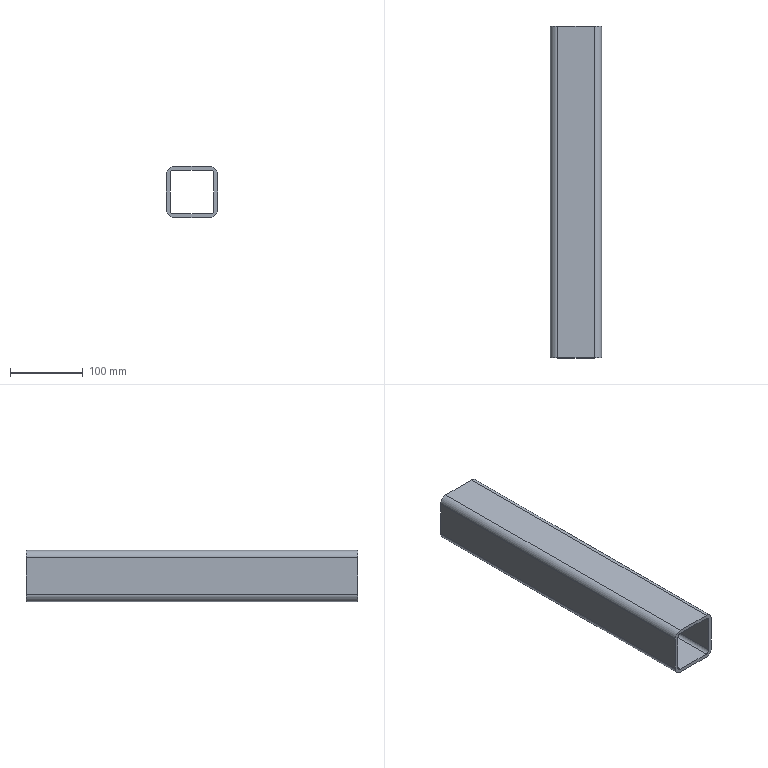Part | SolidWorks | features WeldMemberFeat 1, WeldmentFeature 1 | 1 solid | 18 faces | box 70 x 455 x 70 mm | volume 562207 mm3 | plane 10 | cylinder 8 | commonest cylinder face diameters 10 x4 20 x4
STEP:
#1=CARTESIAN_POINT('',(-35.,0.,25.));
#2=VERTEX_POINT('',#1);
#3=CARTESIAN_POINT('',(-25.,0.,35.));
#4=VERTEX_POINT('',#3);
#5=CARTESIAN_POINT('',(-25.,0.,25.));
#6=DIRECTION('',(0.,1.,0.));
#7=DIRECTION('',(0.,0.,1.));
#8=AXIS2_PLACEMENT_3D('',#5,#6,#7);
#9=CIRCLE('',#8,10.);
#10=EDGE_CURVE('',#2,#4,#9,.T.);
#11=ORIENTED_EDGE('',*,*,#10,.T.);
#12=CARTESIAN_POINT('',(-25.,455.,35.));
#13=VERTEX_POINT('',#12);
#14=CARTESIAN_POINT('',(-25.,455.,35.));
#15=DIRECTION('',(0.,-1.,0.));
#16=VECTOR('',#15,1000.);
#17=LINE('',#14,#16);
#18=EDGE_CURVE('',#13,#4,#17,.T.);
#19=ORIENTED_EDGE('',*,*,#18,.F.);
#20=CARTESIAN_POINT('',(-35.,455.,25.));
#21=VERTEX_POINT('',#20);
#22=CARTESIAN_POINT('',(-25.,455.,25.));
#23=DIRECTION('',(0.,1.,0.));
#24=DIRECTION('',(0.,0.,1.));
#25=AXIS2_PLACEMENT_3D('',#22,#23,#24);
#26=CIRCLE('',#25,10.);
#27=EDGE_CURVE('',#21,#13,#26,.T.);
#28=ORIENTED_EDGE('',*,*,#27,.F.);
#29=CARTESIAN_POINT('',(-35.,455.,25.));
#30=DIRECTION('',(0.,-1.,0.));
#31=VECTOR('',#30,1000.);
#32=LINE('',#29,#31);
#33=EDGE_CURVE('',#21,#2,#32,.T.);
#34=ORIENTED_EDGE('',*,*,#33,.T.);
#35=EDGE_LOOP('',(#11,#19,#28,#34));
#36=FACE_OUTER_BOUND('',#35,.T.);
#37=CARTESIAN_POINT('',(-25.,455.,25.));
#38=DIRECTION('',(0.,-1.,0.));
#39=DIRECTION('',(0.,0.,-1.));
#40=AXIS2_PLACEMENT_3D('',#37,#38,#39);
#41=CYLINDRICAL_SURFACE('',#40,10.);
#42=ADVANCED_FACE('',(#36),#41,.T.);
#43=CARTESIAN_POINT('',(25.,0.,35.));
#44=VERTEX_POINT('',#43);
#45=CARTESIAN_POINT('',(-25.,0.,35.));
#46=DIRECTION('',(1.,0.,0.));
#47=VECTOR('',#46,1000.);
#48=LINE('',#45,#47);
#49=EDGE_CURVE('',#4,#44,#48,.T.);
#50=ORIENTED_EDGE('',*,*,#49,.T.);
#51=CARTESIAN_POINT('',(25.,455.,35.));
#52=VERTEX_POINT('',#51);
#53=CARTESIAN_POINT('',(25.,455.,35.));
#54=DIRECTION('',(0.,-1.,0.));
#55=VECTOR('',#54,1000.);
#56=LINE('',#53,#55);
#57=EDGE_CURVE('',#52,#44,#56,.T.);
#58=ORIENTED_EDGE('',*,*,#57,.F.);
#59=CARTESIAN_POINT('',(-25.,455.,35.));
#60=DIRECTION('',(1.,0.,0.));
#61=VECTOR('',#60,1000.);
#62=LINE('',#59,#61);
#63=EDGE_CURVE('',#13,#52,#62,.T.);
#64=ORIENTED_EDGE('',*,*,#63,.F.);
#65=ORIENTED_EDGE('',*,*,#18,.T.);
#66=EDGE_LOOP('',(#50,#58,#64,#65));
#67=FACE_OUTER_BOUND('',#66,.T.);
#68=CARTESIAN_POINT('',(-25.,455.,35.));
#69=DIRECTION('',(0.,0.,-1.));
#70=DIRECTION('',(-1.,0.,0.));
#71=AXIS2_PLACEMENT_3D('',#68,#69,#70);
#72=PLANE('',#71);
#73=ADVANCED_FACE('',(#67),#72,.F.);
#74=CARTESIAN_POINT('',(35.,0.,25.));
#75=VERTEX_POINT('',#74);
#76=CARTESIAN_POINT('',(25.,0.,25.));
#77=DIRECTION('',(0.,1.,0.));
#78=DIRECTION('',(0.,0.,1.));
#79=AXIS2_PLACEMENT_3D('',#76,#77,#78);
#80=CIRCLE('',#79,10.);
#81=EDGE_CURVE('',#44,#75,#80,.T.);
#82=ORIENTED_EDGE('',*,*,#81,.T.);
#83=CARTESIAN_POINT('',(35.,455.,25.));
#84=VERTEX_POINT('',#83);
#85=CARTESIAN_POINT('',(35.,455.,25.));
#86=DIRECTION('',(0.,-1.,0.));
#87=VECTOR('',#86,1000.);
#88=LINE('',#85,#87);
#89=EDGE_CURVE('',#84,#75,#88,.T.);
#90=ORIENTED_EDGE('',*,*,#89,.F.);
#91=CARTESIAN_POINT('',(25.,455.,25.));
#92=DIRECTION('',(0.,1.,0.));
#93=DIRECTION('',(0.,0.,1.));
#94=AXIS2_PLACEMENT_3D('',#91,#92,#93);
#95=CIRCLE('',#94,10.);
#96=EDGE_CURVE('',#52,#84,#95,.T.);
#97=ORIENTED_EDGE('',*,*,#96,.F.);
#98=ORIENTED_EDGE('',*,*,#57,.T.);
#99=EDGE_LOOP('',(#82,#90,#97,#98));
#100=FACE_OUTER_BOUND('',#99,.T.);
#101=CARTESIAN_POINT('',(25.,455.,25.));
#102=DIRECTION('',(0.,-1.,0.));
#103=DIRECTION('',(0.,0.,-1.));
#104=AXIS2_PLACEMENT_3D('',#101,#102,#103);
#105=CYLINDRICAL_SURFACE('',#104,10.);
#106=ADVANCED_FACE('',(#100),#105,.T.);
#107=CARTESIAN_POINT('',(35.,0.,-25.));
#108=VERTEX_POINT('',#107);
#109=CARTESIAN_POINT('',(35.,0.,-25.));
#110=DIRECTION('',(0.,0.,-1.));
#111=VECTOR('',#110,1000.);
#112=LINE('',#109,#111);
#113=EDGE_CURVE('',#75,#108,#112,.T.);
#114=ORIENTED_EDGE('',*,*,#113,.T.);
#115=CARTESIAN_POINT('',(35.,455.,-25.));
#116=VERTEX_POINT('',#115);
#117=CARTESIAN_POINT('',(35.,455.,-25.));
#118=DIRECTION('',(0.,-1.,0.));
#119=VECTOR('',#118,1000.);
#120=LINE('',#117,#119);
#121=EDGE_CURVE('',#116,#108,#120,.T.);
#122=ORIENTED_EDGE('',*,*,#121,.F.);
#123=CARTESIAN_POINT('',(35.,455.,-25.));
#124=DIRECTION('',(0.,0.,-1.));
#125=VECTOR('',#124,1000.);
#126=LINE('',#123,#125);
#127=EDGE_CURVE('',#84,#116,#126,.T.);
#128=ORIENTED_EDGE('',*,*,#127,.F.);
#129=ORIENTED_EDGE('',*,*,#89,.T.);
#130=EDGE_LOOP('',(#114,#122,#128,#129));
#131=FACE_OUTER_BOUND('',#130,.T.);
#132=CARTESIAN_POINT('',(35.,455.,-25.));
#133=DIRECTION('',(-1.,0.,0.));
#134=DIRECTION('',(0.,0.,1.));
#135=AXIS2_PLACEMENT_3D('',#132,#133,#134);
#136=PLANE('',#135);
#137=ADVANCED_FACE('',(#131),#136,.F.);
#138=CARTESIAN_POINT('',(25.,0.,-35.));
#139=VERTEX_POINT('',#138);
#140=CARTESIAN_POINT('',(25.,0.,-25.));
#141=DIRECTION('',(0.,1.,0.));
#142=DIRECTION('',(0.,0.,1.));
#143=AXIS2_PLACEMENT_3D('',#140,#141,#142);
#144=CIRCLE('',#143,10.);
#145=EDGE_CURVE('',#108,#139,#144,.T.);
#146=ORIENTED_EDGE('',*,*,#145,.T.);
#147=CARTESIAN_POINT('',(25.,455.,-35.));
#148=VERTEX_POINT('',#147);
#149=CARTESIAN_POINT('',(25.,455.,-35.));
#150=DIRECTION('',(0.,-1.,0.));
#151=VECTOR('',#150,1000.);
#152=LINE('',#149,#151);
#153=EDGE_CURVE('',#148,#139,#152,.T.);
#154=ORIENTED_EDGE('',*,*,#153,.F.);
#155=CARTESIAN_POINT('',(25.,455.,-25.));
#156=DIRECTION('',(0.,1.,0.));
#157=DIRECTION('',(0.,0.,1.));
#158=AXIS2_PLACEMENT_3D('',#155,#156,#157);
#159=CIRCLE('',#158,10.);
#160=EDGE_CURVE('',#116,#148,#159,.T.);
#161=ORIENTED_EDGE('',*,*,#160,.F.);
#162=ORIENTED_EDGE('',*,*,#121,.T.);
#163=EDGE_LOOP('',(#146,#154,#161,#162));
#164=FACE_OUTER_BOUND('',#163,.T.);
#165=CARTESIAN_POINT('',(25.,455.,-25.));
#166=DIRECTION('',(0.,-1.,0.));
#167=DIRECTION('',(0.,0.,-1.));
#168=AXIS2_PLACEMENT_3D('',#165,#166,#167);
#169=CYLINDRICAL_SURFACE('',#168,10.);
#170=ADVANCED_FACE('',(#164),#169,.T.);
#171=CARTESIAN_POINT('',(-25.,0.,-35.));
#172=VERTEX_POINT('',#171);
#173=CARTESIAN_POINT('',(25.,0.,-35.));
#174=DIRECTION('',(-1.,0.,0.));
#175=VECTOR('',#174,1000.);
#176=LINE('',#173,#175);
#177=EDGE_CURVE('',#139,#172,#176,.T.);
#178=ORIENTED_EDGE('',*,*,#177,.T.);
#179=CARTESIAN_POINT('',(-25.,455.,-35.));
#180=VERTEX_POINT('',#179);
#181=CARTESIAN_POINT('',(-25.,455.,-35.));
#182=DIRECTION('',(0.,-1.,0.));
#183=VECTOR('',#182,1000.);
#184=LINE('',#181,#183);
#185=EDGE_CURVE('',#180,#172,#184,.T.);
#186=ORIENTED_EDGE('',*,*,#185,.F.);
#187=CARTESIAN_POINT('',(25.,455.,-35.));
#188=DIRECTION('',(-1.,0.,0.));
#189=VECTOR('',#188,1000.);
#190=LINE('',#187,#189);
#191=EDGE_CURVE('',#148,#180,#190,.T.);
#192=ORIENTED_EDGE('',*,*,#191,.F.);
#193=ORIENTED_EDGE('',*,*,#153,.T.);
#194=EDGE_LOOP('',(#178,#186,#192,#193));
#195=FACE_OUTER_BOUND('',#194,.T.);
#196=CARTESIAN_POINT('',(25.,455.,-35.));
#197=DIRECTION('',(0.,0.,1.));
#198=DIRECTION('',(1.,0.,0.));
#199=AXIS2_PLACEMENT_3D('',#196,#197,#198);
#200=PLANE('',#199);
#201=ADVANCED_FACE('',(#195),#200,.F.);
#202=CARTESIAN_POINT('',(-35.,0.,-25.));
#203=VERTEX_POINT('',#202);
#204=CARTESIAN_POINT('',(-25.,0.,-25.));
#205=DIRECTION('',(0.,1.,0.));
#206=DIRECTION('',(0.,0.,1.));
#207=AXIS2_PLACEMENT_3D('',#204,#205,#206);
#208=CIRCLE('',#207,10.);
#209=EDGE_CURVE('',#172,#203,#208,.T.);
#210=ORIENTED_EDGE('',*,*,#209,.T.);
#211=CARTESIAN_POINT('',(-35.,455.,-25.));
#212=VERTEX_POINT('',#211);
#213=CARTESIAN_POINT('',(-35.,455.,-25.));
#214=DIRECTION('',(0.,-1.,0.));
#215=VECTOR('',#214,1000.);
#216=LINE('',#213,#215);
#217=EDGE_CURVE('',#212,#203,#216,.T.);
#218=ORIENTED_EDGE('',*,*,#217,.F.);
#219=CARTESIAN_POINT('',(-25.,455.,-25.));
#220=DIRECTION('',(0.,1.,0.));
#221=DIRECTION('',(0.,0.,1.));
#222=AXIS2_PLACEMENT_3D('',#219,#220,#221);
#223=CIRCLE('',#222,10.);
#224=EDGE_CURVE('',#180,#212,#223,.T.);
#225=ORIENTED_EDGE('',*,*,#224,.F.);
#226=ORIENTED_EDGE('',*,*,#185,.T.);
#227=EDGE_LOOP('',(#210,#218,#225,#226));
#228=FACE_OUTER_BOUND('',#227,.T.);
#229=CARTESIAN_POINT('',(-25.,455.,-25.));
#230=DIRECTION('',(0.,-1.,0.));
#231=DIRECTION('',(0.,0.,-1.));
#232=AXIS2_PLACEMENT_3D('',#229,#230,#231);
#233=CYLINDRICAL_SURFACE('',#232,10.);
#234=ADVANCED_FACE('',(#228),#233,.T.);
#235=CARTESIAN_POINT('',(25.,0.,30.));
#236=VERTEX_POINT('',#235);
#237=CARTESIAN_POINT('',(30.,0.,25.));
#238=VERTEX_POINT('',#237);
#239=CARTESIAN_POINT('',(25.,0.,25.));
#240=DIRECTION('',(0.,1.,0.));
#241=DIRECTION('',(0.,0.,1.));
#242=AXIS2_PLACEMENT_3D('',#239,#240,#241);
#243=CIRCLE('',#242,5.);
#244=EDGE_CURVE('',#236,#238,#243,.T.);
#245=ORIENTED_EDGE('',*,*,#244,.F.);
#246=CARTESIAN_POINT('',(25.,455.,30.));
#247=VERTEX_POINT('',#246);
#248=CARTESIAN_POINT('',(25.,455.,30.));
#249=DIRECTION('',(0.,-1.,0.));
#250=VECTOR('',#249,1000.);
#251=LINE('',#248,#250);
#252=EDGE_CURVE('',#247,#236,#251,.T.);
#253=ORIENTED_EDGE('',*,*,#252,.F.);
#254=CARTESIAN_POINT('',(30.,455.,25.));
#255=VERTEX_POINT('',#254);
#256=CARTESIAN_POINT('',(25.,455.,25.));
#257=DIRECTION('',(0.,1.,0.));
#258=DIRECTION('',(0.,0.,1.));
#259=AXIS2_PLACEMENT_3D('',#256,#257,#258);
#260=CIRCLE('',#259,5.);
#261=EDGE_CURVE('',#247,#255,#260,.T.);
#262=ORIENTED_EDGE('',*,*,#261,.T.);
#263=CARTESIAN_POINT('',(30.,455.,25.));
#264=DIRECTION('',(0.,-1.,0.));
#265=VECTOR('',#264,1000.);
#266=LINE('',#263,#265);
#267=EDGE_CURVE('',#255,#238,#266,.T.);
#268=ORIENTED_EDGE('',*,*,#267,.T.);
#269=EDGE_LOOP('',(#245,#253,#262,#268));
#270=FACE_OUTER_BOUND('',#269,.T.);
#271=CARTESIAN_POINT('',(25.,455.,25.));
#272=DIRECTION('',(0.,-1.,0.));
#273=DIRECTION('',(0.,0.,-1.));
#274=AXIS2_PLACEMENT_3D('',#271,#272,#273);
#275=CYLINDRICAL_SURFACE('',#274,5.);
#276=ADVANCED_FACE('',(#270),#275,.F.);
#277=CARTESIAN_POINT('',(-25.,0.,30.));
#278=VERTEX_POINT('',#277);
#279=CARTESIAN_POINT('',(-25.,0.,30.));
#280=DIRECTION('',(1.,0.,0.));
#281=VECTOR('',#280,1000.);
#282=LINE('',#279,#281);
#283=EDGE_CURVE('',#278,#236,#282,.T.);
#284=ORIENTED_EDGE('',*,*,#283,.F.);
#285=CARTESIAN_POINT('',(-25.,455.,30.));
#286=VERTEX_POINT('',#285);
#287=CARTESIAN_POINT('',(-25.,455.,30.));
#288=DIRECTION('',(0.,-1.,0.));
#289=VECTOR('',#288,1000.);
#290=LINE('',#287,#289);
#291=EDGE_CURVE('',#286,#278,#290,.T.);
#292=ORIENTED_EDGE('',*,*,#291,.F.);
#293=CARTESIAN_POINT('',(-25.,455.,30.));
#294=DIRECTION('',(1.,0.,0.));
#295=VECTOR('',#294,1000.);
#296=LINE('',#293,#295);
#297=EDGE_CURVE('',#286,#247,#296,.T.);
#298=ORIENTED_EDGE('',*,*,#297,.T.);
#299=ORIENTED_EDGE('',*,*,#252,.T.);
#300=EDGE_LOOP('',(#284,#292,#298,#299));
#301=FACE_OUTER_BOUND('',#300,.T.);
#302=CARTESIAN_POINT('',(-25.,455.,30.));
#303=DIRECTION('',(0.,0.,-1.));
#304=DIRECTION('',(-1.,0.,0.));
#305=AXIS2_PLACEMENT_3D('',#302,#303,#304);
#306=PLANE('',#305);
#307=ADVANCED_FACE('',(#301),#306,.T.);
#308=CARTESIAN_POINT('',(-30.,0.,25.));
#309=VERTEX_POINT('',#308);
#310=CARTESIAN_POINT('',(-25.,0.,25.));
#311=DIRECTION('',(0.,1.,0.));
#312=DIRECTION('',(0.,0.,1.));
#313=AXIS2_PLACEMENT_3D('',#310,#311,#312);
#314=CIRCLE('',#313,5.);
#315=EDGE_CURVE('',#309,#278,#314,.T.);
#316=ORIENTED_EDGE('',*,*,#315,.F.);
#317=CARTESIAN_POINT('',(-30.,455.,25.));
#318=VERTEX_POINT('',#317);
#319=CARTESIAN_POINT('',(-30.,455.,25.));
#320=DIRECTION('',(0.,-1.,0.));
#321=VECTOR('',#320,1000.);
#322=LINE('',#319,#321);
#323=EDGE_CURVE('',#318,#309,#322,.T.);
#324=ORIENTED_EDGE('',*,*,#323,.F.);
#325=CARTESIAN_POINT('',(-25.,455.,25.));
#326=DIRECTION('',(0.,1.,0.));
#327=DIRECTION('',(0.,0.,1.));
#328=AXIS2_PLACEMENT_3D('',#325,#326,#327);
#329=CIRCLE('',#328,5.);
#330=EDGE_CURVE('',#318,#286,#329,.T.);
#331=ORIENTED_EDGE('',*,*,#330,.T.);
#332=ORIENTED_EDGE('',*,*,#291,.T.);
#333=EDGE_LOOP('',(#316,#324,#331,#332));
#334=FACE_OUTER_BOUND('',#333,.T.);
#335=CARTESIAN_POINT('',(-25.,455.,25.));
#336=DIRECTION('',(0.,-1.,0.));
#337=DIRECTION('',(0.,0.,-1.));
#338=AXIS2_PLACEMENT_3D('',#335,#336,#337);
#339=CYLINDRICAL_SURFACE('',#338,5.);
#340=ADVANCED_FACE('',(#334),#339,.F.);
#341=CARTESIAN_POINT('',(-30.,0.,-25.));
#342=VERTEX_POINT('',#341);
#343=CARTESIAN_POINT('',(-30.,0.,25.));
#344=DIRECTION('',(0.,0.,1.));
#345=VECTOR('',#344,1000.);
#346=LINE('',#343,#345);
#347=EDGE_CURVE('',#342,#309,#346,.T.);
#348=ORIENTED_EDGE('',*,*,#347,.F.);
#349=CARTESIAN_POINT('',(-30.,455.,-25.));
#350=VERTEX_POINT('',#349);
#351=CARTESIAN_POINT('',(-30.,455.,-25.));
#352=DIRECTION('',(0.,-1.,0.));
#353=VECTOR('',#352,1000.);
#354=LINE('',#351,#353);
#355=EDGE_CURVE('',#350,#342,#354,.T.);
#356=ORIENTED_EDGE('',*,*,#355,.F.);
#357=CARTESIAN_POINT('',(-30.,455.,25.));
#358=DIRECTION('',(0.,0.,1.));
#359=VECTOR('',#358,1000.);
#360=LINE('',#357,#359);
#361=EDGE_CURVE('',#350,#318,#360,.T.);
#362=ORIENTED_EDGE('',*,*,#361,.T.);
#363=ORIENTED_EDGE('',*,*,#323,.T.);
#364=EDGE_LOOP('',(#348,#356,#362,#363));
#365=FACE_OUTER_BOUND('',#364,.T.);
#366=CARTESIAN_POINT('',(-30.,455.,25.));
#367=DIRECTION('',(1.,0.,0.));
#368=DIRECTION('',(0.,0.,-1.));
#369=AXIS2_PLACEMENT_3D('',#366,#367,#368);
#370=PLANE('',#369);
#371=ADVANCED_FACE('',(#365),#370,.T.);
#372=CARTESIAN_POINT('',(-25.,0.,-30.));
#373=VERTEX_POINT('',#372);
#374=CARTESIAN_POINT('',(-25.,0.,-25.));
#375=DIRECTION('',(0.,1.,0.));
#376=DIRECTION('',(0.,0.,1.));
#377=AXIS2_PLACEMENT_3D('',#374,#375,#376);
#378=CIRCLE('',#377,5.);
#379=EDGE_CURVE('',#373,#342,#378,.T.);
#380=ORIENTED_EDGE('',*,*,#379,.F.);
#381=CARTESIAN_POINT('',(-25.,455.,-30.));
#382=VERTEX_POINT('',#381);
#383=CARTESIAN_POINT('',(-25.,455.,-30.));
#384=DIRECTION('',(0.,-1.,0.));
#385=VECTOR('',#384,1000.);
#386=LINE('',#383,#385);
#387=EDGE_CURVE('',#382,#373,#386,.T.);
#388=ORIENTED_EDGE('',*,*,#387,.F.);
#389=CARTESIAN_POINT('',(-25.,455.,-25.));
#390=DIRECTION('',(0.,1.,0.));
#391=DIRECTION('',(0.,0.,1.));
#392=AXIS2_PLACEMENT_3D('',#389,#390,#391);
#393=CIRCLE('',#392,5.);
#394=EDGE_CURVE('',#382,#350,#393,.T.);
#395=ORIENTED_EDGE('',*,*,#394,.T.);
#396=ORIENTED_EDGE('',*,*,#355,.T.);
#397=EDGE_LOOP('',(#380,#388,#395,#396));
#398=FACE_OUTER_BOUND('',#397,.T.);
#399=CARTESIAN_POINT('',(-25.,455.,-25.));
#400=DIRECTION('',(0.,-1.,0.));
#401=DIRECTION('',(0.,0.,-1.));
#402=AXIS2_PLACEMENT_3D('',#399,#400,#401);
#403=CYLINDRICAL_SURFACE('',#402,5.);
#404=ADVANCED_FACE('',(#398),#403,.F.);
#405=CARTESIAN_POINT('',(25.,0.,-30.));
#406=VERTEX_POINT('',#405);
#407=CARTESIAN_POINT('',(25.,0.,-30.));
#408=DIRECTION('',(-1.,0.,0.));
#409=VECTOR('',#408,1000.);
#410=LINE('',#407,#409);
#411=EDGE_CURVE('',#406,#373,#410,.T.);
#412=ORIENTED_EDGE('',*,*,#411,.F.);
#413=CARTESIAN_POINT('',(25.,455.,-30.));
#414=VERTEX_POINT('',#413);
#415=CARTESIAN_POINT('',(25.,455.,-30.));
#416=DIRECTION('',(0.,-1.,0.));
#417=VECTOR('',#416,1000.);
#418=LINE('',#415,#417);
#419=EDGE_CURVE('',#414,#406,#418,.T.);
#420=ORIENTED_EDGE('',*,*,#419,.F.);
#421=CARTESIAN_POINT('',(25.,455.,-30.));
#422=DIRECTION('',(-1.,0.,0.));
#423=VECTOR('',#422,1000.);
#424=LINE('',#421,#423);
#425=EDGE_CURVE('',#414,#382,#424,.T.);
#426=ORIENTED_EDGE('',*,*,#425,.T.);
#427=ORIENTED_EDGE('',*,*,#387,.T.);
#428=EDGE_LOOP('',(#412,#420,#426,#427));
#429=FACE_OUTER_BOUND('',#428,.T.);
#430=CARTESIAN_POINT('',(25.,455.,-30.));
#431=DIRECTION('',(0.,0.,1.));
#432=DIRECTION('',(1.,0.,0.));
#433=AXIS2_PLACEMENT_3D('',#430,#431,#432);
#434=PLANE('',#433);
#435=ADVANCED_FACE('',(#429),#434,.T.);
#436=CARTESIAN_POINT('',(30.,0.,-25.));
#437=VERTEX_POINT('',#436);
#438=CARTESIAN_POINT('',(25.,0.,-25.));
#439=DIRECTION('',(0.,1.,0.));
#440=DIRECTION('',(0.,0.,1.));
#441=AXIS2_PLACEMENT_3D('',#438,#439,#440);
#442=CIRCLE('',#441,5.);
#443=EDGE_CURVE('',#437,#406,#442,.T.);
#444=ORIENTED_EDGE('',*,*,#443,.F.);
#445=CARTESIAN_POINT('',(30.,455.,-25.));
#446=VERTEX_POINT('',#445);
#447=CARTESIAN_POINT('',(30.,455.,-25.));
#448=DIRECTION('',(0.,-1.,0.));
#449=VECTOR('',#448,1000.);
#450=LINE('',#447,#449);
#451=EDGE_CURVE('',#446,#437,#450,.T.);
#452=ORIENTED_EDGE('',*,*,#451,.F.);
#453=CARTESIAN_POINT('',(25.,455.,-25.));
#454=DIRECTION('',(0.,1.,0.));
#455=DIRECTION('',(0.,0.,1.));
#456=AXIS2_PLACEMENT_3D('',#453,#454,#455);
#457=CIRCLE('',#456,5.);
#458=EDGE_CURVE('',#446,#414,#457,.T.);
#459=ORIENTED_EDGE('',*,*,#458,.T.);
#460=ORIENTED_EDGE('',*,*,#419,.T.);
#461=EDGE_LOOP('',(#444,#452,#459,#460));
#462=FACE_OUTER_BOUND('',#461,.T.);
#463=CARTESIAN_POINT('',(25.,455.,-25.));
#464=DIRECTION('',(0.,-1.,0.));
#465=DIRECTION('',(0.,0.,-1.));
#466=AXIS2_PLACEMENT_3D('',#463,#464,#465);
#467=CYLINDRICAL_SURFACE('',#466,5.);
#468=ADVANCED_FACE('',(#462),#467,.F.);
#469=CARTESIAN_POINT('',(30.,0.,-25.));
#470=DIRECTION('',(0.,0.,-1.));
#471=VECTOR('',#470,1000.);
#472=LINE('',#469,#471);
#473=EDGE_CURVE('',#238,#437,#472,.T.);
#474=ORIENTED_EDGE('',*,*,#473,.F.);
#475=ORIENTED_EDGE('',*,*,#267,.F.);
#476=CARTESIAN_POINT('',(30.,455.,-25.));
#477=DIRECTION('',(0.,0.,-1.));
#478=VECTOR('',#477,1000.);
#479=LINE('',#476,#478);
#480=EDGE_CURVE('',#255,#446,#479,.T.);
#481=ORIENTED_EDGE('',*,*,#480,.T.);
#482=ORIENTED_EDGE('',*,*,#451,.T.);
#483=EDGE_LOOP('',(#474,#475,#481,#482));
#484=FACE_OUTER_BOUND('',#483,.T.);
#485=CARTESIAN_POINT('',(30.,455.,-25.));
#486=DIRECTION('',(-1.,0.,0.));
#487=DIRECTION('',(0.,0.,1.));
#488=AXIS2_PLACEMENT_3D('',#485,#486,#487);
#489=PLANE('',#488);
#490=ADVANCED_FACE('',(#484),#489,.T.);
#491=CARTESIAN_POINT('',(-35.,0.,25.));
#492=DIRECTION('',(0.,0.,1.));
#493=VECTOR('',#492,1000.);
#494=LINE('',#491,#493);
#495=EDGE_CURVE('',#203,#2,#494,.T.);
#496=ORIENTED_EDGE('',*,*,#495,.T.);
#497=ORIENTED_EDGE('',*,*,#33,.F.);
#498=CARTESIAN_POINT('',(-35.,455.,25.));
#499=DIRECTION('',(0.,0.,1.));
#500=VECTOR('',#499,1000.);
#501=LINE('',#498,#500);
#502=EDGE_CURVE('',#212,#21,#501,.T.);
#503=ORIENTED_EDGE('',*,*,#502,.F.);
#504=ORIENTED_EDGE('',*,*,#217,.T.);
#505=EDGE_LOOP('',(#496,#497,#503,#504));
#506=FACE_OUTER_BOUND('',#505,.T.);
#507=CARTESIAN_POINT('',(-35.,455.,25.));
#508=DIRECTION('',(1.,0.,0.));
#509=DIRECTION('',(0.,0.,-1.));
#510=AXIS2_PLACEMENT_3D('',#507,#508,#509);
#511=PLANE('',#510);
#512=ADVANCED_FACE('',(#506),#511,.F.);
#513=ORIENTED_EDGE('',*,*,#261,.F.);
#514=ORIENTED_EDGE('',*,*,#297,.F.);
#515=ORIENTED_EDGE('',*,*,#330,.F.);
#516=ORIENTED_EDGE('',*,*,#361,.F.);
#517=ORIENTED_EDGE('',*,*,#394,.F.);
#518=ORIENTED_EDGE('',*,*,#425,.F.);
#519=ORIENTED_EDGE('',*,*,#458,.F.);
#520=ORIENTED_EDGE('',*,*,#480,.F.);
#521=EDGE_LOOP('',(#513,#514,#515,#516,#517,#518,#519,#520));
#522=FACE_BOUND('',#521,.T.);
#523=ORIENTED_EDGE('',*,*,#27,.T.);
#524=ORIENTED_EDGE('',*,*,#63,.T.);
#525=ORIENTED_EDGE('',*,*,#96,.T.);
#526=ORIENTED_EDGE('',*,*,#127,.T.);
#527=ORIENTED_EDGE('',*,*,#160,.T.);
#528=ORIENTED_EDGE('',*,*,#191,.T.);
#529=ORIENTED_EDGE('',*,*,#224,.T.);
#530=ORIENTED_EDGE('',*,*,#502,.T.);
#531=EDGE_LOOP('',(#523,#524,#525,#526,#527,#528,#529,#530));
#532=FACE_OUTER_BOUND('',#531,.T.);
#533=CARTESIAN_POINT('',(-25.,455.,25.));
#534=DIRECTION('',(0.,1.,0.));
#535=DIRECTION('',(0.,0.,1.));
#536=AXIS2_PLACEMENT_3D('',#533,#534,#535);
#537=PLANE('',#536);
#538=ADVANCED_FACE('',(#522,#532),#537,.T.);
#539=ORIENTED_EDGE('',*,*,#244,.T.);
#540=ORIENTED_EDGE('',*,*,#473,.T.);
#541=ORIENTED_EDGE('',*,*,#443,.T.);
#542=ORIENTED_EDGE('',*,*,#411,.T.);
#543=ORIENTED_EDGE('',*,*,#379,.T.);
#544=ORIENTED_EDGE('',*,*,#347,.T.);
#545=ORIENTED_EDGE('',*,*,#315,.T.);
#546=ORIENTED_EDGE('',*,*,#283,.T.);
#547=EDGE_LOOP('',(#539,#540,#541,#542,#543,#544,#545,#546));
#548=FACE_BOUND('',#547,.T.);
#549=ORIENTED_EDGE('',*,*,#10,.F.);
#550=ORIENTED_EDGE('',*,*,#495,.F.);
#551=ORIENTED_EDGE('',*,*,#209,.F.);
#552=ORIENTED_EDGE('',*,*,#177,.F.);
#553=ORIENTED_EDGE('',*,*,#145,.F.);
#554=ORIENTED_EDGE('',*,*,#113,.F.);
#555=ORIENTED_EDGE('',*,*,#81,.F.);
#556=ORIENTED_EDGE('',*,*,#49,.F.);
#557=EDGE_LOOP('',(#549,#550,#551,#552,#553,#554,#555,#556));
#558=FACE_OUTER_BOUND('',#557,.T.);
#559=CARTESIAN_POINT('',(-25.,0.,25.));
#560=DIRECTION('',(0.,1.,0.));
#561=DIRECTION('',(0.,0.,1.));
#562=AXIS2_PLACEMENT_3D('',#559,#560,#561);
#563=PLANE('',#562);
#564=ADVANCED_FACE('',(#548,#558),#563,.F.);
#565=CLOSED_SHELL('',(#42,#73,#106,#137,#170,#201,#234,#276,#307,#340,#371,#404,#435,#468,#490,#512,#538,#564));
#566=MANIFOLD_SOLID_BREP('',#565);
#567=CARTESIAN_POINT('',(0.,0.,0.));
#568=DIRECTION('',(0.,0.,1.));
#569=DIRECTION('',(1.,0.,0.));
#570=AXIS2_PLACEMENT_3D('',#567,#568,#569);
#571=(LENGTH_UNIT()NAMED_UNIT(*)SI_UNIT(.MILLI.,.METRE.));
#572=UNCERTAINTY_MEASURE_WITH_UNIT(LENGTH_MEASURE(0.00001),#571,'','');
#573=(NAMED_UNIT(*)PLANE_ANGLE_UNIT()SI_UNIT($,.RADIAN.));
#574=(NAMED_UNIT(*)SI_UNIT($,.STERADIAN.)SOLID_ANGLE_UNIT());
#575=(GEOMETRIC_REPRESENTATION_CONTEXT(3)GLOBAL_UNCERTAINTY_ASSIGNED_CONTEXT((#572))GLOBAL_UNIT_ASSIGNED_CONTEXT((#571,#573,#574))REPRESENTATION_CONTEXT('',''));
#576=ADVANCED_BREP_SHAPE_REPRESENTATION('',(#566,#570),#575);